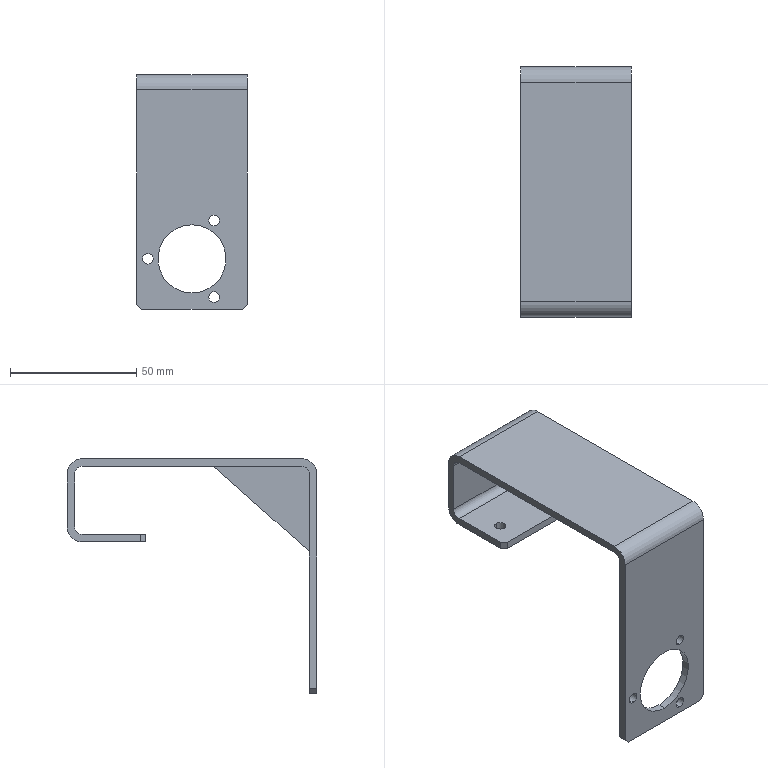Part | STEP file | rotary joint support_SUS304 | 1 solid | 38 faces | box 44 x 99 x 93 mm | volume 31796 mm3 | cylinder 19 | plane 19 | commonest cylinder face diameters 4.2 x6 4.5 x4 6 x4 12 x3 27 x2